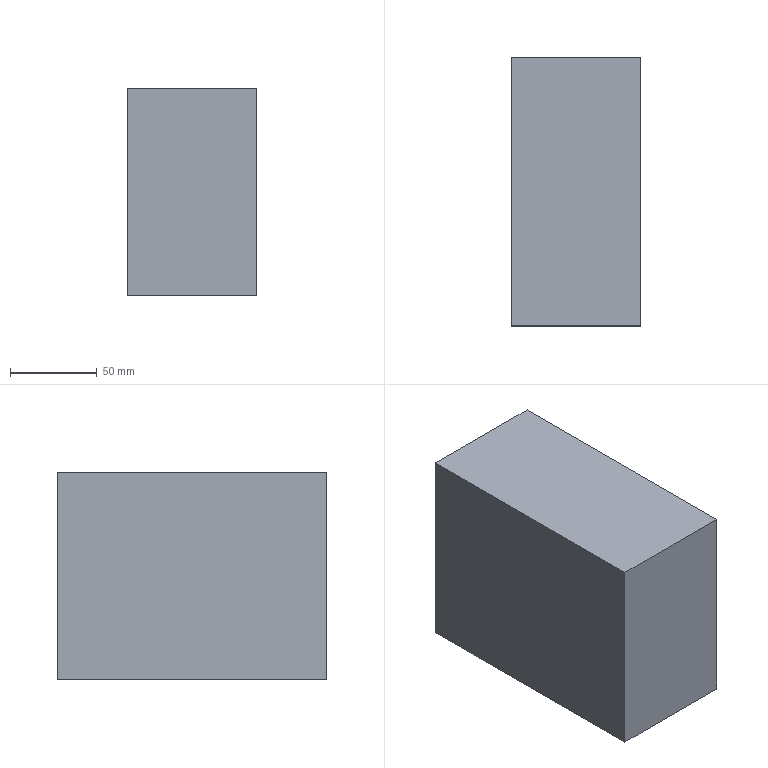Part | NX | features solid 2 | 1 solid | 6 faces | box 75 x 155 x 120 mm | volume 1395000 mm3 | plane 6
STEP:
#1=CARTESIAN_POINT('',(-1485.,-385.,-400.));
#2=VERTEX_POINT('',#1);
#3=CARTESIAN_POINT('',(-1560.,-385.,-400.));
#4=VERTEX_POINT('',#3);
#5=CARTESIAN_POINT('',(-1485.,-385.,-400.));
#6=DIRECTION('',(1.,0.,0.));
#7=VECTOR('',#6,1000.);
#8=LINE('',#5,#7);
#9=EDGE_CURVE('',#2,#4,#8,.F.);
#10=ORIENTED_EDGE('',*,*,#9,.T.);
#11=CARTESIAN_POINT('',(-1560.,-230.,-400.));
#12=VERTEX_POINT('',#11);
#13=CARTESIAN_POINT('',(-1560.,-385.,-400.));
#14=DIRECTION('',(0.,1.,0.));
#15=VECTOR('',#14,1000.);
#16=LINE('',#13,#15);
#17=EDGE_CURVE('',#4,#12,#16,.T.);
#18=ORIENTED_EDGE('',*,*,#17,.T.);
#19=CARTESIAN_POINT('',(-1485.,-230.,-400.));
#20=VERTEX_POINT('',#19);
#21=CARTESIAN_POINT('',(-1485.,-230.,-400.));
#22=DIRECTION('',(1.,0.,0.));
#23=VECTOR('',#22,1000.);
#24=LINE('',#21,#23);
#25=EDGE_CURVE('',#20,#12,#24,.F.);
#26=ORIENTED_EDGE('',*,*,#25,.F.);
#27=CARTESIAN_POINT('',(-1485.,-385.,-400.));
#28=DIRECTION('',(0.,1.,0.));
#29=VECTOR('',#28,1000.);
#30=LINE('',#27,#29);
#31=EDGE_CURVE('',#2,#20,#30,.T.);
#32=ORIENTED_EDGE('',*,*,#31,.F.);
#33=EDGE_LOOP('',(#10,#18,#26,#32));
#34=FACE_BOUND('',#33,.T.);
#35=CARTESIAN_POINT('',(-1485.,-385.,-400.));
#36=DIRECTION('',(0.,0.,-1.));
#37=DIRECTION('',(0.,1.,0.));
#38=AXIS2_PLACEMENT_3D('',#35,#36,#37);
#39=PLANE('',#38);
#40=ADVANCED_FACE('',(#34),#39,.T.);
#41=ORIENTED_EDGE('',*,*,#25,.T.);
#42=CARTESIAN_POINT('',(-1560.,-230.,-280.));
#43=VERTEX_POINT('',#42);
#44=CARTESIAN_POINT('',(-1560.,-230.,-400.));
#45=DIRECTION('',(0.,0.,-1.));
#46=VECTOR('',#45,1000.);
#47=LINE('',#44,#46);
#48=EDGE_CURVE('',#12,#43,#47,.F.);
#49=ORIENTED_EDGE('',*,*,#48,.T.);
#50=CARTESIAN_POINT('',(-1485.,-230.,-280.));
#51=VERTEX_POINT('',#50);
#52=CARTESIAN_POINT('',(-1485.,-230.,-280.));
#53=DIRECTION('',(1.,0.,0.));
#54=VECTOR('',#53,1000.);
#55=LINE('',#52,#54);
#56=EDGE_CURVE('',#51,#43,#55,.F.);
#57=ORIENTED_EDGE('',*,*,#56,.F.);
#58=CARTESIAN_POINT('',(-1485.,-230.,-400.));
#59=DIRECTION('',(0.,0.,1.));
#60=VECTOR('',#59,1000.);
#61=LINE('',#58,#60);
#62=EDGE_CURVE('',#20,#51,#61,.T.);
#63=ORIENTED_EDGE('',*,*,#62,.F.);
#64=EDGE_LOOP('',(#41,#49,#57,#63));
#65=FACE_BOUND('',#64,.T.);
#66=CARTESIAN_POINT('',(-1485.,-230.,-400.));
#67=DIRECTION('',(0.,1.,0.));
#68=DIRECTION('',(0.,0.,1.));
#69=AXIS2_PLACEMENT_3D('',#66,#67,#68);
#70=PLANE('',#69);
#71=ADVANCED_FACE('',(#65),#70,.T.);
#72=ORIENTED_EDGE('',*,*,#56,.T.);
#73=CARTESIAN_POINT('',(-1560.,-385.,-280.));
#74=VERTEX_POINT('',#73);
#75=CARTESIAN_POINT('',(-1560.,-385.,-280.));
#76=DIRECTION('',(0.,1.,0.));
#77=VECTOR('',#76,1000.);
#78=LINE('',#75,#77);
#79=EDGE_CURVE('',#74,#43,#78,.T.);
#80=ORIENTED_EDGE('',*,*,#79,.F.);
#81=CARTESIAN_POINT('',(-1485.,-385.,-280.));
#82=VERTEX_POINT('',#81);
#83=CARTESIAN_POINT('',(-1485.,-385.,-280.));
#84=DIRECTION('',(1.,0.,0.));
#85=VECTOR('',#84,1000.);
#86=LINE('',#83,#85);
#87=EDGE_CURVE('',#82,#74,#86,.F.);
#88=ORIENTED_EDGE('',*,*,#87,.F.);
#89=CARTESIAN_POINT('',(-1485.,-385.,-280.));
#90=DIRECTION('',(0.,1.,0.));
#91=VECTOR('',#90,1000.);
#92=LINE('',#89,#91);
#93=EDGE_CURVE('',#82,#51,#92,.T.);
#94=ORIENTED_EDGE('',*,*,#93,.T.);
#95=EDGE_LOOP('',(#72,#80,#88,#94));
#96=FACE_BOUND('',#95,.T.);
#97=CARTESIAN_POINT('',(-1485.,-385.,-280.));
#98=DIRECTION('',(0.,0.,-1.));
#99=DIRECTION('',(0.,1.,0.));
#100=AXIS2_PLACEMENT_3D('',#97,#98,#99);
#101=PLANE('',#100);
#102=ADVANCED_FACE('',(#96),#101,.F.);
#103=CARTESIAN_POINT('',(-1485.,-385.,-400.));
#104=DIRECTION('',(0.,0.,1.));
#105=VECTOR('',#104,1000.);
#106=LINE('',#103,#105);
#107=EDGE_CURVE('',#2,#82,#106,.T.);
#108=ORIENTED_EDGE('',*,*,#107,.T.);
#109=ORIENTED_EDGE('',*,*,#87,.T.);
#110=CARTESIAN_POINT('',(-1560.,-385.,-400.));
#111=DIRECTION('',(0.,0.,-1.));
#112=VECTOR('',#111,1000.);
#113=LINE('',#110,#112);
#114=EDGE_CURVE('',#4,#74,#113,.F.);
#115=ORIENTED_EDGE('',*,*,#114,.F.);
#116=ORIENTED_EDGE('',*,*,#9,.F.);
#117=EDGE_LOOP('',(#108,#109,#115,#116));
#118=FACE_BOUND('',#117,.T.);
#119=CARTESIAN_POINT('',(-1485.,-385.,-400.));
#120=DIRECTION('',(0.,1.,0.));
#121=DIRECTION('',(0.,0.,1.));
#122=AXIS2_PLACEMENT_3D('',#119,#120,#121);
#123=PLANE('',#122);
#124=ADVANCED_FACE('',(#118),#123,.F.);
#125=ORIENTED_EDGE('',*,*,#79,.T.);
#126=ORIENTED_EDGE('',*,*,#48,.F.);
#127=ORIENTED_EDGE('',*,*,#17,.F.);
#128=ORIENTED_EDGE('',*,*,#114,.T.);
#129=EDGE_LOOP('',(#125,#126,#127,#128));
#130=FACE_BOUND('',#129,.T.);
#131=CARTESIAN_POINT('',(-1560.,-385.,-400.));
#132=DIRECTION('',(1.,0.,0.));
#133=DIRECTION('',(0.,0.,-1.));
#134=AXIS2_PLACEMENT_3D('',#131,#132,#133);
#135=PLANE('',#134);
#136=ADVANCED_FACE('',(#130),#135,.F.);
#137=ORIENTED_EDGE('',*,*,#93,.F.);
#138=ORIENTED_EDGE('',*,*,#107,.F.);
#139=ORIENTED_EDGE('',*,*,#31,.T.);
#140=ORIENTED_EDGE('',*,*,#62,.T.);
#141=EDGE_LOOP('',(#137,#138,#139,#140));
#142=FACE_BOUND('',#141,.T.);
#143=CARTESIAN_POINT('',(-1485.,-385.,-400.));
#144=DIRECTION('',(1.,0.,0.));
#145=DIRECTION('',(0.,0.,-1.));
#146=AXIS2_PLACEMENT_3D('',#143,#144,#145);
#147=PLANE('',#146);
#148=ADVANCED_FACE('',(#142),#147,.T.);
#149=CLOSED_SHELL('',(#40,#71,#102,#124,#136,#148));
#150=MANIFOLD_SOLID_BREP('',#149);
#151=(LENGTH_UNIT()NAMED_UNIT(*)SI_UNIT(.MILLI.,.METRE.));
#152=UNCERTAINTY_MEASURE_WITH_UNIT(LENGTH_MEASURE(0.00001),#151,'','');
#153=(NAMED_UNIT(*)PLANE_ANGLE_UNIT()SI_UNIT($,.RADIAN.));
#154=(NAMED_UNIT(*)SI_UNIT($,.STERADIAN.)SOLID_ANGLE_UNIT());
#155=(GEOMETRIC_REPRESENTATION_CONTEXT(3)GLOBAL_UNCERTAINTY_ASSIGNED_CONTEXT((#152))GLOBAL_UNIT_ASSIGNED_CONTEXT((#151,#153,#154))REPRESENTATION_CONTEXT('',''));
#156=ADVANCED_BREP_SHAPE_REPRESENTATION('',(#150),#155);